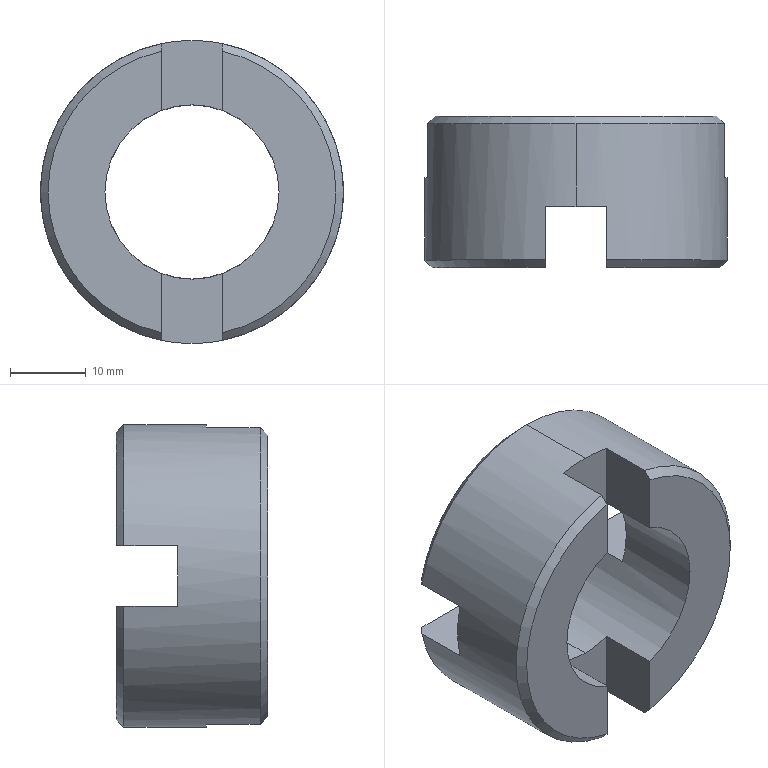Part | STEP file | CON-009 | 1 solid | 25 faces | box 40 x 20 x 40 mm | volume 14486 mm3 | plane 16 | cone 5 | cylinder 4 | commonest cylinder face diameters 23 x2 40 x2